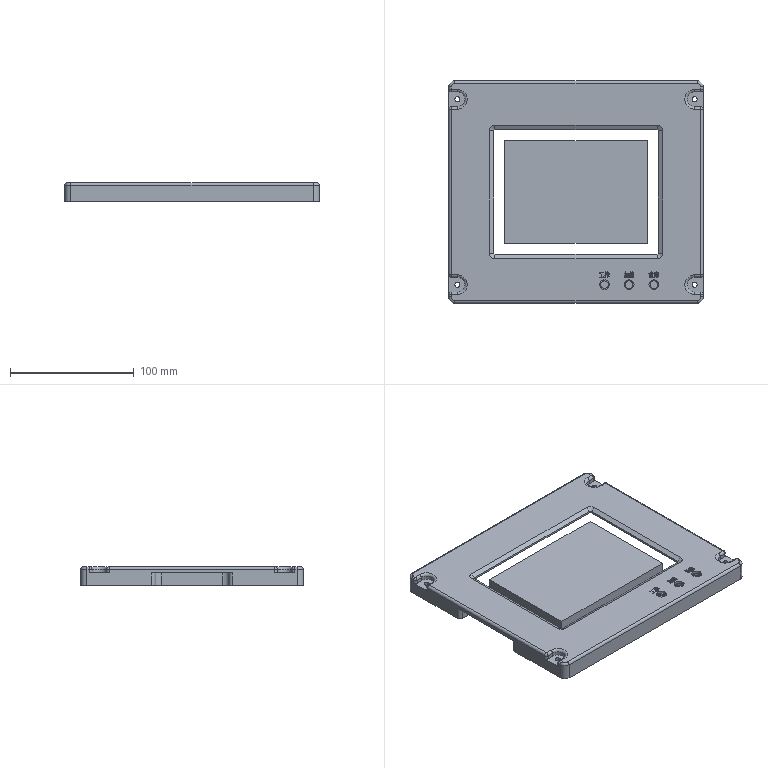CAM job | Mastercam | 3-axis milling, 5-axis milling, drilling | part box 206 x 180 x 15 mm | stock box 211 x 190 x 15 mm
Tools:
tool_number,name,type,diameter_mm,corner_radius_mm,flutes,flute_length_mm,overall_length_mm,shoulder_length_mm,holder_diameter_mm,length_offset,diameter_offset,default_rpm,default_feed_mm_min,default_plunge_mm_min,coolant
1,4 Bull Nose Mill,bull end mill,4,1,4,25,100,25,50,1,1,10000,4000,600,COOL_OFF
1,4 Bull Nose Mill,bull end mill,4,1,4,4,8,4.8,50,1,1,10000,4000,600,COOL_OFF
2,2 Flat End Mill,end mill,2,0,4,25,75,25,50,2,2,10000,3000,600,COOL_OFF
4,4 Flat End Mill,end mill,4,0,4,25,75,25,50,4,4,1000,3000,600,COOL_OFF
5,4 Chamfer Mill,chamfer mill,4,0,4,25,75,30,50,5,5,3000,300,600,COOL_OFF
8,8 Flat End Mill,end mill,8,0,4,25,75,25,50,8,8,7000,3000,600,COOL_OFF
9,10 Flat End Mill,end mill,10,0,4,25,75,25,50,9,9,7000,3000,600,COOL_OFF
10,10 Flat End Mill,end mill,10,0,4,25,75,25,50,10,10,7000,1000,600,COOL_OFF
14,2 Ball Mill / Bull Nose Mill,ball end mill,2,1,4,25,100,30,50,14,14,11000,3000,600,COOL_OFF
24,100 Flat End Mill,end mill,100,0,4,25,75,25,50,24,24,4000,1000,600,COOL_OFF
Operations:
seq,operation,operation_type,tool_number,tool_name,tool_diameter_mm,spindle_rpm,feed_mm_min,plunge_mm_min,retract_mm_min,cycle_time_s,wcs,posted,nc_file
1,Facing - [WCS: Plane] - [Tplane: Plane],Facing,24,100 Flat End Mill,100,4000,1000,600,1200,232.084,Plane,yes,.nc
2,Contour (Ramp) - [WCS: Plane] - [Tplane: Plane],Contour,9,10 Flat End Mill,10,7000,3000,600,1200,254.602,Plane,yes,.nc
3,Contour (Ramp) - [WCS: Plane] - [Tplane: Plane],Contour,9,10 Flat End Mill,10,7000,3000,600,1200,36.553,Plane,yes,.nc
4,Contour (2D) - [WCS: Plane] - [Tplane: Plane],Contour,10,10 Flat End Mill,10,7000,1000,600,1200,14.063,Plane,yes,.nc
5,Contour (2D) - [WCS: Plane] - [Tplane: Plane],Contour,10,10 Flat End Mill,10,7000,1000,600,1200,50.14,Plane,yes,.nc
6,Surface Finish Flowline - [WCS: Plane] - [Tplane: Plane],MultiSurfaceFinishFlowline,1,4 Bull Nose Mill,4,10000,4000,600,1200,86.583,Plane,yes,.nc
7,Unified Morph - [WCS: Plane] - [Tplane: Plane],461,1,4 Bull Nose Mill,4,10000,4000,600,1200,369.242,Plane,yes,.nc
8,Surface Finish Flowline - [WCS: Plane] - [Tplane: Plane],MultiSurfaceFinishFlowline,14,2 Ball Mill / Bull Nose Mill,2,11000,2000,600,1200,585.895,Plane,yes,.nc
9,Helix Bore - [WCS: Plane] - [Tplane: Plane],HelixBore,4,4 Flat End Mill,4,10000,3000,600,1200,28.585,Plane,yes,.nc
10,Contour (Ramp) - [WCS: Plane] - [Tplane: Plane],Contour,8,8 Flat End Mill,8,7000,3000,600,1200,25.491,Plane,yes,.nc
11,Drill/Counterbore - [WCS: Plane] - [Tplane: Plane],Drill,5,4 Chamfer Mill,4,3000,300,600,1200,3.274,Plane,yes,.nc
12,Contour (2D chamfer) - [WCS: Plane] - [Tplane: Plane],Contour,5,4 Chamfer Mill,4,7000,1000,600,1200,12.059,Plane,yes,.nc
13,Contour (2D chamfer) - [WCS: Plane] - [Tplane: Plane],Contour,5,4 Chamfer Mill,4,7000,1000,600,1200,5.307,Plane,yes,.nc
14,Facing - [WCS: Plane] - [Tplane: Plane],Facing,24,100 Flat End Mill,100,4000,1000,600,1200,76.202,Plane,yes,.nc
15,2D High Speed (2D Area Mill) - [WCS: Plane-1] - [Tplane: Plane-1],HighSpeed2D,8,8 Flat End Mill,8,7000,3000,600,1200,162.968,Plane-1,yes,.nc
16,Contour (2D) - [WCS: Plane-1] - [Tplane: Plane-1],Contour,8,8 Flat End Mill,8,7000,1000,600,1200,14.436,Plane-1,yes,.nc
17,3D High Speed (Area roughing) - [WCS: Plane-1] - [Tplane: Plane-1],HighSpeed3D,8,8 Flat End Mill,8,8000,4000,600,1200,1547.366,Plane-1,yes,.nc
18,Helix Bore - [WCS: Plane-1] - [Tplane: Plane-1],HelixBore,4,4 Flat End Mill,4,10000,3000,600,1200,38.39,Plane-1,yes,.nc
19,3D High Speed (Waterline rest passes) - [WCS: Plane-1] - [Tplane: Plane-1],HighSpeed3D,4,4 Flat End Mill,4,10000,3000,600,1200,103.422,Plane-1,yes,.nc
20,3D High Speed (Horizontal) - [WCS: Plane-1] - [Tplane: Plane-1],HighSpeed3D,4,4 Flat End Mill,4,7000,1000,600,1200,890.032,Plane-1,yes,.nc
21,3D High Speed (Waterline) - [WCS: Plane-1] - [Tplane: Plane-1],HighSpeed3D,4,4 Flat End Mill,4,10000,1000,600,1200,385.299,Plane-1,yes,.nc
22,Drill/Counterbore - [WCS: Plane-1] - [Tplane: Plane-1],Drill,5,4 Chamfer Mill,4,3000,300,600,1200,3.274,Plane-1,yes,.nc
23,Model Chamfer - [WCS: Plane-1] - [Tplane: Plane-1],ModelChamfer,5,4 Chamfer Mill,4,7000,1000,600,1200,176.35,Plane-1,yes,.nc
24,Manual Entry (Cl),ManualEntry,,,,0,0,0,0,0,Plane-1,yes,.nc
25,Manual Entry (M00),ManualEntry,,,,0,0,0,0,0,Plane-1,yes,.nc
26,Contour (Ramp) - [WCS: Plane-1] - [Tplane: Plane-1],Contour,2,2 Flat End Mill,2,10000,3000,600,1200,78.927,Plane-1,yes,.nc
27,Contour (2D) - [WCS: Plane-1] - [Tplane: Plane-1],Contour,2,2 Flat End Mill,2,10000,500,600,1200,56.215,Plane-1,yes,.nc
28,Contour (2D chamfer) - [WCS: Plane-1] - [Tplane: Plane-1],Contour,5,4 Chamfer Mill,4,10000,1000,600,1200,28.613,Plane-1,yes,.nc